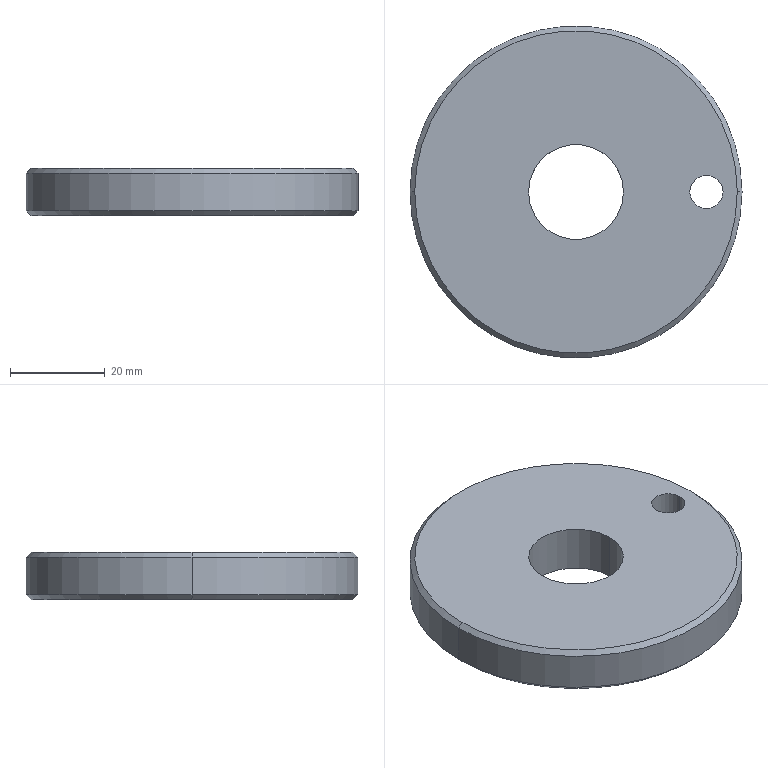Part | SolidWorks | features ICE 2, Chamfer 1, Extrusion 1 | 1 solid | 12 faces | box 70 x 70 x 10 mm | volume 34740 mm3 | cylinder 6 | cone 4 | plane 2 | commonest cylinder face diameters 7 x2 20 x2 70 x2
STEP:
#1=CARTESIAN_POINT('',(24.,0.,0.));
#2=VERTEX_POINT('',#1);
#3=CARTESIAN_POINT('',(31.,0.,0.));
#4=VERTEX_POINT('',#3);
#5=CARTESIAN_POINT('',(27.5,0.,0.));
#6=DIRECTION('',(0.,0.,1.));
#7=DIRECTION('',(1.,0.,0.));
#8=AXIS2_PLACEMENT_3D('',#5,#6,#7);
#9=CIRCLE('',#8,3.5);
#10=EDGE_CURVE('',#2,#4,#9,.T.);
#11=ORIENTED_EDGE('',*,*,#10,.F.);
#12=CARTESIAN_POINT('',(24.,0.,10.));
#13=VERTEX_POINT('',#12);
#14=CARTESIAN_POINT('',(24.,0.,-19.));
#15=DIRECTION('',(0.,0.,1.));
#16=VECTOR('',#15,1000.);
#17=LINE('',#14,#16);
#18=EDGE_CURVE('',#2,#13,#17,.T.);
#19=ORIENTED_EDGE('',*,*,#18,.T.);
#20=CARTESIAN_POINT('',(31.,0.,10.));
#21=VERTEX_POINT('',#20);
#22=CARTESIAN_POINT('',(27.5,0.,10.));
#23=DIRECTION('',(0.,0.,1.));
#24=DIRECTION('',(1.,0.,0.));
#25=AXIS2_PLACEMENT_3D('',#22,#23,#24);
#26=CIRCLE('',#25,3.5);
#27=EDGE_CURVE('',#13,#21,#26,.T.);
#28=ORIENTED_EDGE('',*,*,#27,.T.);
#29=CARTESIAN_POINT('',(31.,0.,-19.));
#30=DIRECTION('',(0.,0.,1.));
#31=VECTOR('',#30,1000.);
#32=LINE('',#29,#31);
#33=EDGE_CURVE('',#4,#21,#32,.T.);
#34=ORIENTED_EDGE('',*,*,#33,.F.);
#35=EDGE_LOOP('',(#11,#19,#28,#34));
#36=FACE_OUTER_BOUND('',#35,.T.);
#37=CARTESIAN_POINT('',(27.5,0.,-19.));
#38=DIRECTION('',(0.,0.,1.));
#39=DIRECTION('',(1.,0.,0.));
#40=AXIS2_PLACEMENT_3D('',#37,#38,#39);
#41=CYLINDRICAL_SURFACE('',#40,3.5);
#42=ADVANCED_FACE('',(#36),#41,.F.);
#43=CARTESIAN_POINT('',(-10.,0.,0.));
#44=VERTEX_POINT('',#43);
#45=CARTESIAN_POINT('',(10.,0.,0.));
#46=VERTEX_POINT('',#45);
#47=CARTESIAN_POINT('',(0.,0.,0.));
#48=DIRECTION('',(0.,0.,1.));
#49=DIRECTION('',(1.,0.,0.));
#50=AXIS2_PLACEMENT_3D('',#47,#48,#49);
#51=CIRCLE('',#50,10.);
#52=EDGE_CURVE('',#44,#46,#51,.T.);
#53=ORIENTED_EDGE('',*,*,#52,.F.);
#54=CARTESIAN_POINT('',(-10.,0.,10.));
#55=VERTEX_POINT('',#54);
#56=CARTESIAN_POINT('',(-10.,0.,-20.));
#57=DIRECTION('',(0.,0.,1.));
#58=VECTOR('',#57,1000.);
#59=LINE('',#56,#58);
#60=EDGE_CURVE('',#44,#55,#59,.T.);
#61=ORIENTED_EDGE('',*,*,#60,.T.);
#62=CARTESIAN_POINT('',(10.,0.,10.));
#63=VERTEX_POINT('',#62);
#64=CARTESIAN_POINT('',(0.,0.,10.));
#65=DIRECTION('',(0.,0.,1.));
#66=DIRECTION('',(1.,0.,0.));
#67=AXIS2_PLACEMENT_3D('',#64,#65,#66);
#68=CIRCLE('',#67,10.);
#69=EDGE_CURVE('',#55,#63,#68,.T.);
#70=ORIENTED_EDGE('',*,*,#69,.T.);
#71=CARTESIAN_POINT('',(10.,0.,-20.));
#72=DIRECTION('',(0.,0.,1.));
#73=VECTOR('',#72,1000.);
#74=LINE('',#71,#73);
#75=EDGE_CURVE('',#46,#63,#74,.T.);
#76=ORIENTED_EDGE('',*,*,#75,.F.);
#77=EDGE_LOOP('',(#53,#61,#70,#76));
#78=FACE_OUTER_BOUND('',#77,.T.);
#79=CARTESIAN_POINT('',(0.,0.,-20.));
#80=DIRECTION('',(0.,0.,1.));
#81=DIRECTION('',(1.,0.,0.));
#82=AXIS2_PLACEMENT_3D('',#79,#80,#81);
#83=CYLINDRICAL_SURFACE('',#82,10.);
#84=ADVANCED_FACE('',(#78),#83,.F.);
#85=CARTESIAN_POINT('',(34.,0.,10.));
#86=VERTEX_POINT('',#85);
#87=CARTESIAN_POINT('',(-34.,0.,10.));
#88=VERTEX_POINT('',#87);
#89=CARTESIAN_POINT('',(0.,0.,10.));
#90=DIRECTION('',(0.,0.,1.));
#91=DIRECTION('',(1.,0.,0.));
#92=AXIS2_PLACEMENT_3D('',#89,#90,#91);
#93=CIRCLE('',#92,34.);
#94=EDGE_CURVE('',#86,#88,#93,.T.);
#95=ORIENTED_EDGE('',*,*,#94,.F.);
#96=CARTESIAN_POINT('',(35.,0.,9.));
#97=VERTEX_POINT('',#96);
#98=CARTESIAN_POINT('',(34.,0.,10.));
#99=DIRECTION('',(0.7071,0.,-0.7071));
#100=VECTOR('',#99,1000.);
#101=LINE('',#98,#100);
#102=EDGE_CURVE('',#86,#97,#101,.T.);
#103=ORIENTED_EDGE('',*,*,#102,.T.);
#104=CARTESIAN_POINT('',(-35.,0.,9.));
#105=VERTEX_POINT('',#104);
#106=CARTESIAN_POINT('',(0.,0.,9.));
#107=DIRECTION('',(0.,0.,-1.));
#108=DIRECTION('',(1.,0.,0.));
#109=AXIS2_PLACEMENT_3D('',#106,#107,#108);
#110=CIRCLE('',#109,35.);
#111=EDGE_CURVE('',#105,#97,#110,.T.);
#112=ORIENTED_EDGE('',*,*,#111,.F.);
#113=CARTESIAN_POINT('',(-34.,0.,10.));
#114=DIRECTION('',(-0.7071,0.,-0.7071));
#115=VECTOR('',#114,1000.);
#116=LINE('',#113,#115);
#117=EDGE_CURVE('',#88,#105,#116,.T.);
#118=ORIENTED_EDGE('',*,*,#117,.F.);
#119=EDGE_LOOP('',(#95,#103,#112,#118));
#120=FACE_OUTER_BOUND('',#119,.T.);
#121=CARTESIAN_POINT('',(0.,0.,10.));
#122=DIRECTION('',(0.,0.,-1.));
#123=DIRECTION('',(-1.,0.,0.));
#124=AXIS2_PLACEMENT_3D('',#121,#122,#123);
#125=CONICAL_SURFACE('',#124,34.,0.7854);
#126=ADVANCED_FACE('',(#120),#125,.T.);
#127=CARTESIAN_POINT('',(-34.,0.,0.));
#128=VERTEX_POINT('',#127);
#129=CARTESIAN_POINT('',(34.,0.,0.));
#130=VERTEX_POINT('',#129);
#131=CARTESIAN_POINT('',(0.,0.,0.));
#132=DIRECTION('',(0.,0.,-1.));
#133=DIRECTION('',(1.,0.,0.));
#134=AXIS2_PLACEMENT_3D('',#131,#132,#133);
#135=CIRCLE('',#134,34.);
#136=EDGE_CURVE('',#128,#130,#135,.T.);
#137=ORIENTED_EDGE('',*,*,#136,.F.);
#138=CARTESIAN_POINT('',(-35.,0.,1.));
#139=VERTEX_POINT('',#138);
#140=CARTESIAN_POINT('',(-35.,0.,1.));
#141=DIRECTION('',(-0.7071,0.,0.7071));
#142=VECTOR('',#141,1000.);
#143=LINE('',#140,#142);
#144=EDGE_CURVE('',#128,#139,#143,.T.);
#145=ORIENTED_EDGE('',*,*,#144,.T.);
#146=CARTESIAN_POINT('',(35.,0.,1.));
#147=VERTEX_POINT('',#146);
#148=CARTESIAN_POINT('',(0.,0.,1.));
#149=DIRECTION('',(0.,0.,1.));
#150=DIRECTION('',(1.,0.,0.));
#151=AXIS2_PLACEMENT_3D('',#148,#149,#150);
#152=CIRCLE('',#151,35.);
#153=EDGE_CURVE('',#147,#139,#152,.T.);
#154=ORIENTED_EDGE('',*,*,#153,.F.);
#155=CARTESIAN_POINT('',(35.,0.,1.));
#156=DIRECTION('',(0.7071,0.,0.7071));
#157=VECTOR('',#156,1000.);
#158=LINE('',#155,#157);
#159=EDGE_CURVE('',#130,#147,#158,.T.);
#160=ORIENTED_EDGE('',*,*,#159,.F.);
#161=EDGE_LOOP('',(#137,#145,#154,#160));
#162=FACE_OUTER_BOUND('',#161,.T.);
#163=CARTESIAN_POINT('',(0.,0.,1.));
#164=DIRECTION('',(0.,0.,1.));
#165=DIRECTION('',(1.,0.,0.));
#166=AXIS2_PLACEMENT_3D('',#163,#164,#165);
#167=CONICAL_SURFACE('',#166,35.,0.7854);
#168=ADVANCED_FACE('',(#162),#167,.T.);
#169=ORIENTED_EDGE('',*,*,#111,.T.);
#170=CARTESIAN_POINT('',(35.,0.,10.));
#171=DIRECTION('',(0.,0.,-1.));
#172=VECTOR('',#171,1000.);
#173=LINE('',#170,#172);
#174=EDGE_CURVE('',#97,#147,#173,.T.);
#175=ORIENTED_EDGE('',*,*,#174,.T.);
#176=ORIENTED_EDGE('',*,*,#153,.T.);
#177=CARTESIAN_POINT('',(-35.,0.,10.));
#178=DIRECTION('',(0.,0.,-1.));
#179=VECTOR('',#178,1000.);
#180=LINE('',#177,#179);
#181=EDGE_CURVE('',#105,#139,#180,.T.);
#182=ORIENTED_EDGE('',*,*,#181,.F.);
#183=EDGE_LOOP('',(#169,#175,#176,#182));
#184=FACE_OUTER_BOUND('',#183,.T.);
#185=CARTESIAN_POINT('',(0.,0.,10.));
#186=DIRECTION('',(0.,0.,-1.));
#187=DIRECTION('',(-1.,0.,0.));
#188=AXIS2_PLACEMENT_3D('',#185,#186,#187);
#189=CYLINDRICAL_SURFACE('',#188,35.);
#190=ADVANCED_FACE('',(#184),#189,.T.);
#191=ORIENTED_EDGE('',*,*,#174,.F.);
#192=CARTESIAN_POINT('',(0.,0.,9.));
#193=DIRECTION('',(0.,0.,-1.));
#194=DIRECTION('',(1.,0.,0.));
#195=AXIS2_PLACEMENT_3D('',#192,#193,#194);
#196=CIRCLE('',#195,35.);
#197=EDGE_CURVE('',#97,#105,#196,.T.);
#198=ORIENTED_EDGE('',*,*,#197,.T.);
#199=ORIENTED_EDGE('',*,*,#181,.T.);
#200=CARTESIAN_POINT('',(0.,0.,1.));
#201=DIRECTION('',(0.,0.,1.));
#202=DIRECTION('',(1.,0.,0.));
#203=AXIS2_PLACEMENT_3D('',#200,#201,#202);
#204=CIRCLE('',#203,35.);
#205=EDGE_CURVE('',#139,#147,#204,.T.);
#206=ORIENTED_EDGE('',*,*,#205,.T.);
#207=EDGE_LOOP('',(#191,#198,#199,#206));
#208=FACE_OUTER_BOUND('',#207,.T.);
#209=CARTESIAN_POINT('',(0.,0.,10.));
#210=DIRECTION('',(0.,0.,-1.));
#211=DIRECTION('',(-1.,0.,0.));
#212=AXIS2_PLACEMENT_3D('',#209,#210,#211);
#213=CYLINDRICAL_SURFACE('',#212,35.);
#214=ADVANCED_FACE('',(#208),#213,.T.);
#215=CARTESIAN_POINT('',(27.5,0.,10.));
#216=DIRECTION('',(0.,0.,1.));
#217=DIRECTION('',(1.,0.,0.));
#218=AXIS2_PLACEMENT_3D('',#215,#216,#217);
#219=CIRCLE('',#218,3.5);
#220=EDGE_CURVE('',#21,#13,#219,.T.);
#221=ORIENTED_EDGE('',*,*,#220,.F.);
#222=ORIENTED_EDGE('',*,*,#27,.F.);
#223=EDGE_LOOP('',(#221,#222));
#224=FACE_BOUND('',#223,.T.);
#225=CARTESIAN_POINT('',(0.,0.,10.));
#226=DIRECTION('',(0.,0.,1.));
#227=DIRECTION('',(1.,0.,0.));
#228=AXIS2_PLACEMENT_3D('',#225,#226,#227);
#229=CIRCLE('',#228,10.);
#230=EDGE_CURVE('',#63,#55,#229,.T.);
#231=ORIENTED_EDGE('',*,*,#230,.F.);
#232=ORIENTED_EDGE('',*,*,#69,.F.);
#233=EDGE_LOOP('',(#231,#232));
#234=FACE_BOUND('',#233,.T.);
#235=CARTESIAN_POINT('',(0.,0.,10.));
#236=DIRECTION('',(0.,0.,1.));
#237=DIRECTION('',(1.,0.,0.));
#238=AXIS2_PLACEMENT_3D('',#235,#236,#237);
#239=CIRCLE('',#238,34.);
#240=EDGE_CURVE('',#88,#86,#239,.T.);
#241=ORIENTED_EDGE('',*,*,#240,.T.);
#242=ORIENTED_EDGE('',*,*,#94,.T.);
#243=EDGE_LOOP('',(#241,#242));
#244=FACE_OUTER_BOUND('',#243,.T.);
#245=CARTESIAN_POINT('',(0.,0.,10.));
#246=DIRECTION('',(0.,0.,1.));
#247=DIRECTION('',(1.,0.,0.));
#248=AXIS2_PLACEMENT_3D('',#245,#246,#247);
#249=PLANE('',#248);
#250=ADVANCED_FACE('',(#224,#234,#244),#249,.T.);
#251=CARTESIAN_POINT('',(27.5,0.,0.));
#252=DIRECTION('',(0.,0.,1.));
#253=DIRECTION('',(1.,0.,0.));
#254=AXIS2_PLACEMENT_3D('',#251,#252,#253);
#255=CIRCLE('',#254,3.5);
#256=EDGE_CURVE('',#4,#2,#255,.T.);
#257=ORIENTED_EDGE('',*,*,#256,.T.);
#258=ORIENTED_EDGE('',*,*,#10,.T.);
#259=EDGE_LOOP('',(#257,#258));
#260=FACE_BOUND('',#259,.T.);
#261=CARTESIAN_POINT('',(0.,0.,0.));
#262=DIRECTION('',(0.,0.,1.));
#263=DIRECTION('',(1.,0.,0.));
#264=AXIS2_PLACEMENT_3D('',#261,#262,#263);
#265=CIRCLE('',#264,10.);
#266=EDGE_CURVE('',#46,#44,#265,.T.);
#267=ORIENTED_EDGE('',*,*,#266,.T.);
#268=ORIENTED_EDGE('',*,*,#52,.T.);
#269=EDGE_LOOP('',(#267,#268));
#270=FACE_BOUND('',#269,.T.);
#271=CARTESIAN_POINT('',(0.,0.,0.));
#272=DIRECTION('',(0.,0.,-1.));
#273=DIRECTION('',(1.,0.,0.));
#274=AXIS2_PLACEMENT_3D('',#271,#272,#273);
#275=CIRCLE('',#274,34.);
#276=EDGE_CURVE('',#130,#128,#275,.T.);
#277=ORIENTED_EDGE('',*,*,#276,.T.);
#278=ORIENTED_EDGE('',*,*,#136,.T.);
#279=EDGE_LOOP('',(#277,#278));
#280=FACE_OUTER_BOUND('',#279,.T.);
#281=CARTESIAN_POINT('',(0.,0.,0.));
#282=DIRECTION('',(0.,0.,1.));
#283=DIRECTION('',(1.,0.,0.));
#284=AXIS2_PLACEMENT_3D('',#281,#282,#283);
#285=PLANE('',#284);
#286=ADVANCED_FACE('',(#260,#270,#280),#285,.F.);
#287=ORIENTED_EDGE('',*,*,#144,.F.);
#288=ORIENTED_EDGE('',*,*,#276,.F.);
#289=ORIENTED_EDGE('',*,*,#159,.T.);
#290=ORIENTED_EDGE('',*,*,#205,.F.);
#291=EDGE_LOOP('',(#287,#288,#289,#290));
#292=FACE_OUTER_BOUND('',#291,.T.);
#293=CARTESIAN_POINT('',(0.,0.,1.));
#294=DIRECTION('',(0.,0.,1.));
#295=DIRECTION('',(1.,0.,0.));
#296=AXIS2_PLACEMENT_3D('',#293,#294,#295);
#297=CONICAL_SURFACE('',#296,35.,0.7854);
#298=ADVANCED_FACE('',(#292),#297,.T.);
#299=ORIENTED_EDGE('',*,*,#102,.F.);
#300=ORIENTED_EDGE('',*,*,#240,.F.);
#301=ORIENTED_EDGE('',*,*,#117,.T.);
#302=ORIENTED_EDGE('',*,*,#197,.F.);
#303=EDGE_LOOP('',(#299,#300,#301,#302));
#304=FACE_OUTER_BOUND('',#303,.T.);
#305=CARTESIAN_POINT('',(0.,0.,10.));
#306=DIRECTION('',(0.,0.,-1.));
#307=DIRECTION('',(-1.,0.,0.));
#308=AXIS2_PLACEMENT_3D('',#305,#306,#307);
#309=CONICAL_SURFACE('',#308,34.,0.7854);
#310=ADVANCED_FACE('',(#304),#309,.T.);
#311=ORIENTED_EDGE('',*,*,#60,.F.);
#312=ORIENTED_EDGE('',*,*,#266,.F.);
#313=ORIENTED_EDGE('',*,*,#75,.T.);
#314=ORIENTED_EDGE('',*,*,#230,.T.);
#315=EDGE_LOOP('',(#311,#312,#313,#314));
#316=FACE_OUTER_BOUND('',#315,.T.);
#317=CARTESIAN_POINT('',(0.,0.,-20.));
#318=DIRECTION('',(0.,0.,1.));
#319=DIRECTION('',(1.,0.,0.));
#320=AXIS2_PLACEMENT_3D('',#317,#318,#319);
#321=CYLINDRICAL_SURFACE('',#320,10.);
#322=ADVANCED_FACE('',(#316),#321,.F.);
#323=ORIENTED_EDGE('',*,*,#18,.F.);
#324=ORIENTED_EDGE('',*,*,#256,.F.);
#325=ORIENTED_EDGE('',*,*,#33,.T.);
#326=ORIENTED_EDGE('',*,*,#220,.T.);
#327=EDGE_LOOP('',(#323,#324,#325,#326));
#328=FACE_OUTER_BOUND('',#327,.T.);
#329=CARTESIAN_POINT('',(27.5,0.,-19.));
#330=DIRECTION('',(0.,0.,1.));
#331=DIRECTION('',(1.,0.,0.));
#332=AXIS2_PLACEMENT_3D('',#329,#330,#331);
#333=CYLINDRICAL_SURFACE('',#332,3.5);
#334=ADVANCED_FACE('',(#328),#333,.F.);
#335=CLOSED_SHELL('',(#42,#84,#126,#168,#190,#214,#250,#286,#298,#310,#322,#334));
#336=MANIFOLD_SOLID_BREP('',#335);
#337=CARTESIAN_POINT('',(0.,0.,0.));
#338=DIRECTION('',(0.,0.,1.));
#339=DIRECTION('',(1.,0.,0.));
#340=AXIS2_PLACEMENT_3D('',#337,#338,#339);
#341=(LENGTH_UNIT()NAMED_UNIT(*)SI_UNIT(.MILLI.,.METRE.));
#342=UNCERTAINTY_MEASURE_WITH_UNIT(LENGTH_MEASURE(0.00001),#341,'','');
#343=(NAMED_UNIT(*)PLANE_ANGLE_UNIT()SI_UNIT($,.RADIAN.));
#344=(NAMED_UNIT(*)SI_UNIT($,.STERADIAN.)SOLID_ANGLE_UNIT());
#345=(GEOMETRIC_REPRESENTATION_CONTEXT(3)GLOBAL_UNCERTAINTY_ASSIGNED_CONTEXT((#342))GLOBAL_UNIT_ASSIGNED_CONTEXT((#341,#343,#344))REPRESENTATION_CONTEXT('',''));
#346=ADVANCED_BREP_SHAPE_REPRESENTATION('',(#336,#340),#345);